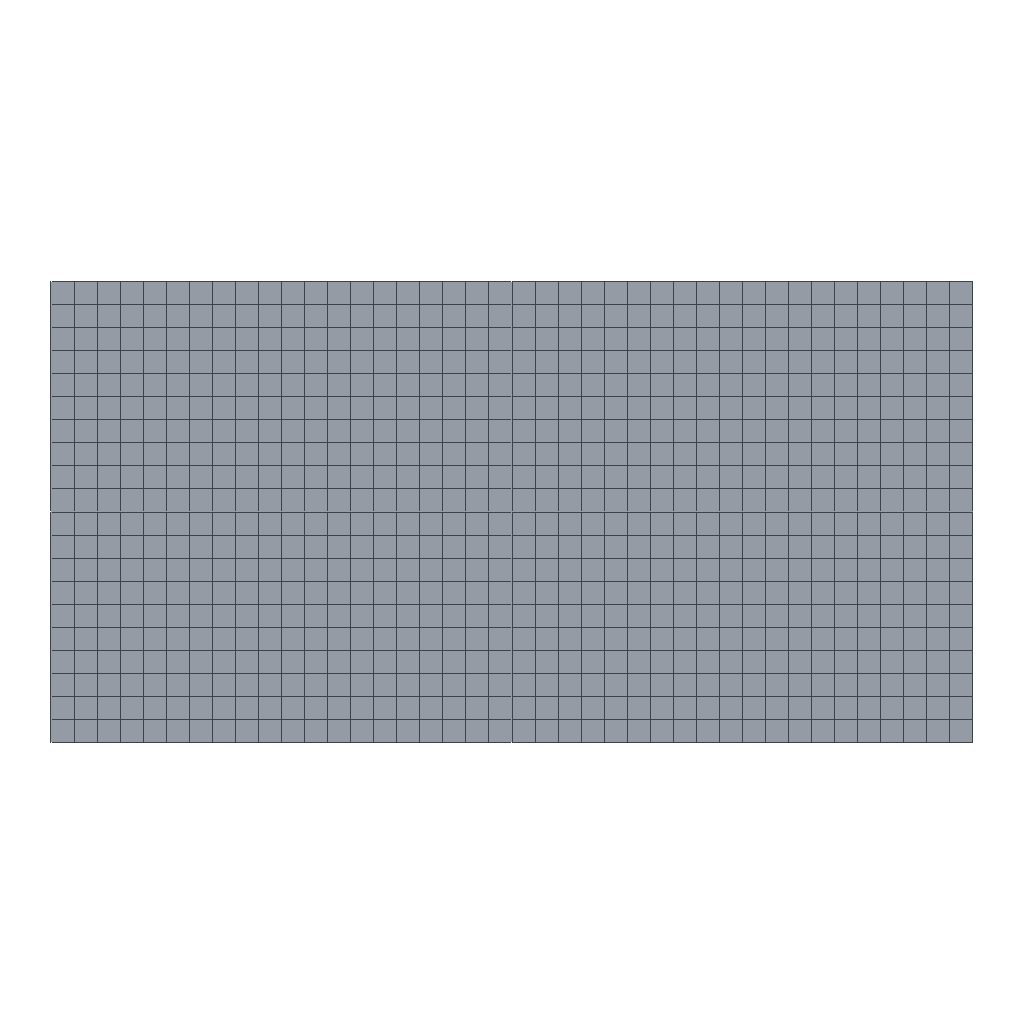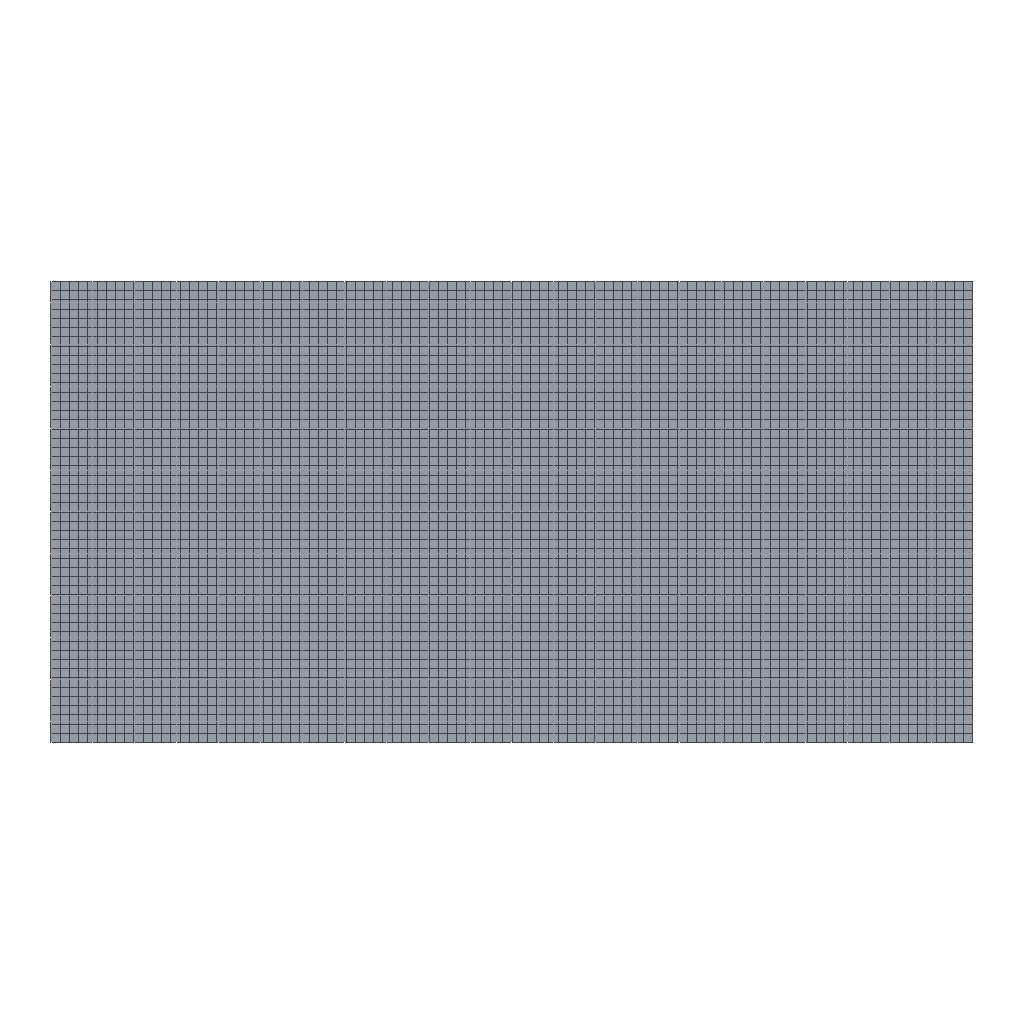Simulation study | abaqus
Set-up summary:
category,name,step,type,value,unit,region
solver,abaqus
solver,version,,,Abaqus/Explicit 3DEXPERIENCE R2017x
solver,version,,,Abaqus/Explicit 6.14-4
units,not stated in the deck,,not stated
analysis,deck1,,transient,transient
load_step,Step-1,Step-1,transient,nlgeom=True
contact,interactions,,,general=0 pairs=1 ties=0
load_step,requested,,,1
mesh,nodes,,,862
mesh,elements,,,800
element_type,CPE4RT,,plane,800
load,load commands in deck,,count,1
bc,support commands in deck,,count,4
analysis,deck2,,transient,transient
load_step,Step-1,Step-1,transient,nlgeom=True
contact,interactions,,,general=0 pairs=1 ties=0
load_step,requested,,,1
mesh,nodes,,,5152
mesh,elements,,,5000
element_type,CPE4RT,,plane,5000
load,load commands in deck,,count,1
bc,support commands in deck,,count,4
material,TC4,,in results
material,TC4,,in results
check,setup vs results,,match,"per instance, exact: element labels, types and connectivity; labels of the nodes the elements use; coordinates of those nodes at SINGLE_PRECISION in 2 of 2 instance(s)"
check,setup vs results,,match,"per instance, exact: element labels, types and connectivity; labels of the nodes the elements use; coordinates of those nodes at SINGLE_PRECISION in 2 of 2 instance(s)"
Abaqus input file, long lists of numbers shortened:
*Heading
** Job name: Job-3 Model name: Model-1
** Generated by: Abaqus/CAE 2017
*Preprint, echo=NO, model=NO, history=NO, contact=NO
**
** PARTS
**
*Part, name=tool
*End Part
**
*Part, name=workpiece
*Node
      1, -0.002,  -1.92086754e-12
      2, -0.002,  -5.00000024e-05
** (859 more lines like these left out)
*Element, type=CPE4RT
  1,   1,   2,  23,  22
  2,   2,   3,  24,  23
** (798 more lines like these left out)
*Nset, nset=Set-5, generate
   1,  861,    1
*Elset, elset=Set-5, generate
   1,  800,    1
*Elset, elset=Set-2
   1,   2,   3,   4,   5,   6,  21,  22,  23,  24,  25,  26,  41,  42,  43,  44
  45,  46,  61,  62,  63,  64,  65,  66,  81,  82,  83,  84,  85,  86, 101, 102
** (13 more lines like these left out)
** Section: Section-TC4
*Solid Section, elset=Set-5, controls=EC-1, material=TC4
0.002,
*End Part
**
**
** ASSEMBLY
**
*Assembly, name=Assembly
**
*Instance, name=tool-1, part=tool
 9.99999999999998e-05,      -0.0002,           0.
*Node
      1, 0.0006, 0.000975,           0.
*Nset, nset=tool-1-RefPt_, internal
1,
*Surface, type=SEGMENTS, name=m_Surf-3
START,           0.,           0.
 LINE, 0.0001197,     0.000975
 LINE, 0.0006,     0.000975
 LINE, 0.0006,  6.30625356458706e-05
 LINE,           0.,           0.
*End Instance
**
*Instance, name=workpiece-1, part=workpiece
*End Instance
**
*Nset, nset=Set-1, instance=tool-1
 1,
*Nset, nset=Set-4, instance=workpiece-1
  19,  20,  21,  40,  41,  42,  61,  62,  63,  82,  83,  84, 103, 104, 105, 124
 125, 126, 145, 146, 147, 166, 167, 168, 187, 188, 189, 208, 209, 210, 229, 230
** (6 more lines like these left out)
*Nset, nset=Set-5, instance=tool-1
 1,
*Nset, nset=Set-7, instance=workpiece-1
   1,   2,   3,   4,   5,   6,  22,  23,  24,  25,  26,  27,  43,  44,  45,  46
  47,  48,  64,  65,  66,  67,  68,  69,  85,  86,  87,  88,  89,  90, 106, 107
** (14 more lines like these left out)
*Nset, nset=_PickedSet14, internal, instance=tool-1
 1,
*Surface, type=NODE, name=Set-7_CNS_, internal
Set-7, 1.
** Constraint: Constraint-1
*Rigid Body, ref node=Set-5, analytical surface=tool-1.m_Surf-3
*End Assembly
**
** ELEMENT CONTROLS
**
*Section Controls, name=EC-1, second order accuracy=YES
1., 1., 1.
*Amplitude, name=Amp-1
             0.,              0.,          0.0001,              1.,          0.0019,              1.,           0.002,              0.
**
** MATERIALS
**
*Material, name=TC4
*Conductivity
  7.5, 20.
  8.7,200.
 11.8,500.
*Damage Initiation, criterion=JOHNSON COOK
 -0.09,  0.25,  -0.5, 0.014,  3.87, 1650.,   25.,    1.
*Damage Evolution, type=DISPLACEMENT
 8e-05,
*Density
4440.,
*Elastic
 1.08e+11, 0.33
*Expansion
 9.1e-06, 20.
 9.2e-06,250.
 9.7e-06,500.
*Inelastic Heat Fraction
         0.9,
*Plastic, hardening=JOHNSON COOK
 8.6e+08, 6.83e+08,     0.47,       1.,    1650.,      25.
*Rate Dependent, type=JOHNSON COOK
 0.035,1.
*Specific Heat
 526.3,
**
** INTERACTION PROPERTIES
**
*Surface Interaction, name=IntProp-1
*Friction
 0.4,
*Surface Behavior, pressure-overclosure=HARD
*Gap Heat Generation
1., 0.5
**
** PREDEFINED FIELDS
**
** Name: Temp works   Type: Temperature
*Initial Conditions, type=TEMPERATURE
_PickedSet14, 298.
** ----------------------------------------------------------------
**
** STEP: Step-1
**
*Step, name=Step-1, nlgeom=YES
*Dynamic, Explicit, adiabatic
, 0.001075
*Bulk Viscosity
0.06, 1.2
** Mass Scaling: Semi-Automatic
**               Whole Model
*Fixed Mass Scaling, factor=200.
**
** BOUNDARY CONDITIONS
**
** Name: BC-1 Type: 速度/角速度
*Boundary, amplitude=Amp-1, type=VELOCITY
Set-5, 1, 1, -2.
Set-5, 2, 2
Set-5, 6, 6
** Name: BC-2 Type: 对称/反对称/完全固定
*Boundary
Set-4, ENCASTRE
**
** INTERACTIONS
**
** Interaction: Int-1
*Contact Pair, interaction=IntProp-1, mechanical constraint=KINEMATIC, cpset=Int-1
tool-1.m_Surf-3, Set-7_CNS_
**
** OUTPUT REQUESTS
**
*Restart, write, number interval=1, time marks=NO
**
** FIELD OUTPUT: F-Output-1
**
*Output, field, number interval=100
*Node Output
A, RF, U, V
*Element Output, directions=YES
EVF, LE, PE, PEEQ, PEEQVAVG, PEVAVG, S, STATUS, SVAVG
*Contact Output
CSTRESS,
**
** HISTORY OUTPUT: H-Output-1
**
*Output, history, time interval=1.075e-05
*Node Output, nset=Set-1
RF1, RF2, RF3, RM, RM1, RM2, RM3, RT
*End Step
Results summary:
result,step,Step-1,completed,increments=12651 time=0.001075/0.001075
result,analysis,,,transient
result,last_loadstep,,,1
result,analysis steps,,count,1
result,primary field,,,U
result,reaction total,,FX,-8.694,model units
result,reaction total,,FY,-22.712,model units
result,reaction total,,FZ,0.0,model units
result,step,cutting,completed,increments=76627 time=0.001075/0.001075
result,analysis,,,transient
result,last_loadstep,,,1
result,analysis steps,,count,1
result,primary field,,,U
result,reaction total,,FX,131.815,model units
result,reaction total,,FY,24.306,model units
result,reaction total,,FZ,0.0,model units